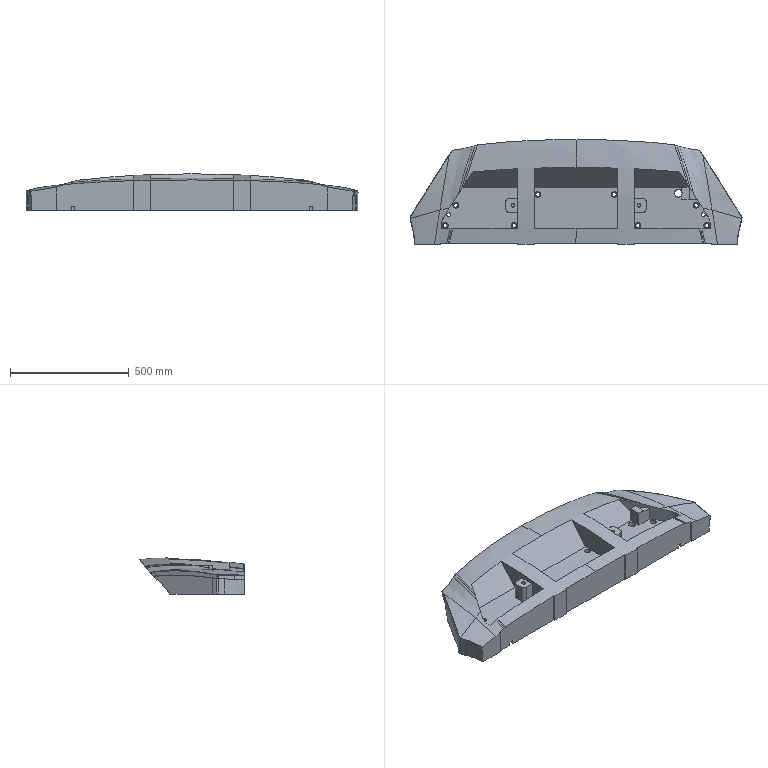Part | NX | features solid 2 | 1 solid | 214 faces | box 1395 x 441.012 x 151.899 mm | volume 42556154 mm3 | plane 95 | spline 78 | cylinder 39 | cone 2 | commonest cylinder face diameters 25 x14 17 x8 20 x8 16 x4 30 x4 32 x1